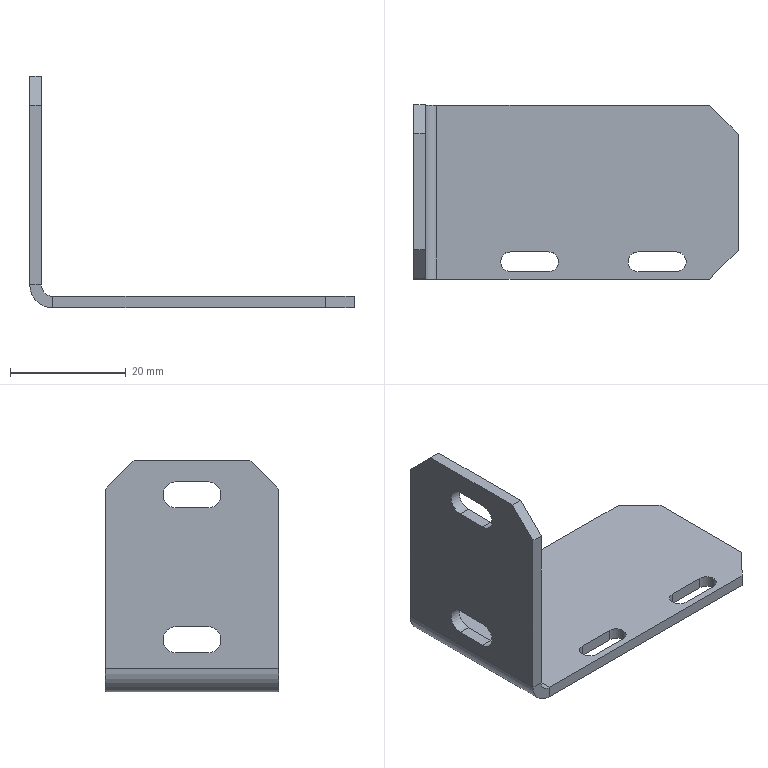Part | SolidWorks | features HoleWzd 2, Chamfer 1, EdgeFlange 1, FlatPattern 1, SMBaseFlange 1, SheetMetal 1 | 1 solid | 34 faces | box 56 x 30 x 40 mm | volume 5174 mm3 | plane 24 | cylinder 10 | commonest cylinder face diameters 3.4 x4 4.5 x4 4 x1 8 x1
STEP:
#1=CARTESIAN_POINT('',(54.,10.,-20.));
#2=VERTEX_POINT('',#1);
#3=CARTESIAN_POINT('',(54.,-10.,-20.));
#4=VERTEX_POINT('',#3);
#5=CARTESIAN_POINT('',(54.,0.,-20.));
#6=DIRECTION('',(0.,-1.,0.));
#7=VECTOR('',#6,1000.);
#8=LINE('',#5,#7);
#9=EDGE_CURVE('',#2,#4,#8,.T.);
#10=ORIENTED_EDGE('',*,*,#9,.T.);
#11=CARTESIAN_POINT('',(49.,-15.,-20.));
#12=VERTEX_POINT('',#11);
#13=CARTESIAN_POINT('',(49.,-15.,-20.));
#14=DIRECTION('',(-0.7071,-0.7071,0.));
#15=VECTOR('',#14,1000.);
#16=LINE('',#13,#15);
#17=EDGE_CURVE('',#4,#12,#16,.T.);
#18=ORIENTED_EDGE('',*,*,#17,.T.);
#19=CARTESIAN_POINT('',(2.,-15.,-20.));
#20=VERTEX_POINT('',#19);
#21=CARTESIAN_POINT('',(0.,-15.,-20.));
#22=DIRECTION('',(-1.,0.,0.));
#23=VECTOR('',#22,1000.);
#24=LINE('',#21,#23);
#25=EDGE_CURVE('',#12,#20,#24,.T.);
#26=ORIENTED_EDGE('',*,*,#25,.T.);
#27=CARTESIAN_POINT('',(2.,15.,-20.));
#28=VERTEX_POINT('',#27);
#29=CARTESIAN_POINT('',(2.,-15.,-20.));
#30=DIRECTION('',(0.,-1.,0.));
#31=VECTOR('',#30,1000.);
#32=LINE('',#29,#31);
#33=EDGE_CURVE('',#28,#20,#32,.T.);
#34=ORIENTED_EDGE('',*,*,#33,.F.);
#35=CARTESIAN_POINT('',(49.,15.,-20.));
#36=VERTEX_POINT('',#35);
#37=CARTESIAN_POINT('',(0.,15.,-20.));
#38=DIRECTION('',(1.,0.,0.));
#39=VECTOR('',#38,1000.);
#40=LINE('',#37,#39);
#41=EDGE_CURVE('',#28,#36,#40,.T.);
#42=ORIENTED_EDGE('',*,*,#41,.T.);
#43=CARTESIAN_POINT('',(54.,10.,-20.));
#44=DIRECTION('',(0.7071,-0.7071,0.));
#45=VECTOR('',#44,1000.);
#46=LINE('',#43,#45);
#47=EDGE_CURVE('',#36,#2,#46,.T.);
#48=ORIENTED_EDGE('',*,*,#47,.T.);
#49=EDGE_LOOP('',(#10,#18,#26,#34,#42,#48));
#50=FACE_OUTER_BOUND('',#49,.T.);
#51=CARTESIAN_POINT('',(21.3,-10.3,-20.));
#52=VERTEX_POINT('',#51);
#53=CARTESIAN_POINT('',(21.3,-13.7,-20.));
#54=VERTEX_POINT('',#53);
#55=CARTESIAN_POINT('',(21.3,-12.,-20.));
#56=DIRECTION('',(0.,0.,-1.));
#57=DIRECTION('',(0.,1.,0.));
#58=AXIS2_PLACEMENT_3D('',#55,#56,#57);
#59=CIRCLE('',#58,1.7);
#60=EDGE_CURVE('',#52,#54,#59,.T.);
#61=ORIENTED_EDGE('',*,*,#60,.F.);
#62=CARTESIAN_POINT('',(14.7,-10.3,-20.));
#63=VERTEX_POINT('',#62);
#64=CARTESIAN_POINT('',(21.3,-10.3,-20.));
#65=DIRECTION('',(-1.,0.,0.));
#66=VECTOR('',#65,1000.);
#67=LINE('',#64,#66);
#68=EDGE_CURVE('',#52,#63,#67,.T.);
#69=ORIENTED_EDGE('',*,*,#68,.T.);
#70=CARTESIAN_POINT('',(14.7,-13.7,-20.));
#71=VERTEX_POINT('',#70);
#72=CARTESIAN_POINT('',(14.7,-12.,-20.));
#73=DIRECTION('',(0.,0.,-1.));
#74=DIRECTION('',(0.,1.,0.));
#75=AXIS2_PLACEMENT_3D('',#72,#73,#74);
#76=CIRCLE('',#75,1.7);
#77=EDGE_CURVE('',#71,#63,#76,.T.);
#78=ORIENTED_EDGE('',*,*,#77,.F.);
#79=CARTESIAN_POINT('',(21.3,-13.7,-20.));
#80=DIRECTION('',(-1.,0.,0.));
#81=VECTOR('',#80,1000.);
#82=LINE('',#79,#81);
#83=EDGE_CURVE('',#54,#71,#82,.T.);
#84=ORIENTED_EDGE('',*,*,#83,.F.);
#85=EDGE_LOOP('',(#61,#69,#78,#84));
#86=FACE_BOUND('',#85,.T.);
#87=CARTESIAN_POINT('',(43.3,-13.7,-20.));
#88=VERTEX_POINT('',#87);
#89=CARTESIAN_POINT('',(36.7,-13.7,-20.));
#90=VERTEX_POINT('',#89);
#91=CARTESIAN_POINT('',(43.3,-13.7,-20.));
#92=DIRECTION('',(-1.,0.,0.));
#93=VECTOR('',#92,1000.);
#94=LINE('',#91,#93);
#95=EDGE_CURVE('',#88,#90,#94,.T.);
#96=ORIENTED_EDGE('',*,*,#95,.F.);
#97=CARTESIAN_POINT('',(43.3,-10.3,-20.));
#98=VERTEX_POINT('',#97);
#99=CARTESIAN_POINT('',(43.3,-12.,-20.));
#100=DIRECTION('',(0.,0.,-1.));
#101=DIRECTION('',(0.,1.,0.));
#102=AXIS2_PLACEMENT_3D('',#99,#100,#101);
#103=CIRCLE('',#102,1.7);
#104=EDGE_CURVE('',#98,#88,#103,.T.);
#105=ORIENTED_EDGE('',*,*,#104,.F.);
#106=CARTESIAN_POINT('',(36.7,-10.3,-20.));
#107=VERTEX_POINT('',#106);
#108=CARTESIAN_POINT('',(43.3,-10.3,-20.));
#109=DIRECTION('',(-1.,0.,0.));
#110=VECTOR('',#109,1000.);
#111=LINE('',#108,#110);
#112=EDGE_CURVE('',#98,#107,#111,.T.);
#113=ORIENTED_EDGE('',*,*,#112,.T.);
#114=CARTESIAN_POINT('',(36.7,-12.,-20.));
#115=DIRECTION('',(0.,0.,-1.));
#116=DIRECTION('',(0.,1.,0.));
#117=AXIS2_PLACEMENT_3D('',#114,#115,#116);
#118=CIRCLE('',#117,1.7);
#119=EDGE_CURVE('',#90,#107,#118,.T.);
#120=ORIENTED_EDGE('',*,*,#119,.F.);
#121=EDGE_LOOP('',(#96,#105,#113,#120));
#122=FACE_BOUND('',#121,.T.);
#123=CARTESIAN_POINT('',(0.,0.,-20.));
#124=DIRECTION('',(0.,0.,1.));
#125=DIRECTION('',(1.,0.,0.));
#126=AXIS2_PLACEMENT_3D('',#123,#124,#125);
#127=PLANE('',#126);
#128=ADVANCED_FACE('',(#50,#86,#122),#127,.F.);
#129=CARTESIAN_POINT('',(-2.,15.,-16.));
#130=VERTEX_POINT('',#129);
#131=CARTESIAN_POINT('',(-2.,15.,15.));
#132=VERTEX_POINT('',#131);
#133=CARTESIAN_POINT('',(-2.,15.,20.));
#134=DIRECTION('',(0.,0.,1.));
#135=VECTOR('',#134,1000.);
#136=LINE('',#133,#135);
#137=EDGE_CURVE('',#130,#132,#136,.T.);
#138=ORIENTED_EDGE('',*,*,#137,.T.);
#139=CARTESIAN_POINT('',(0.,15.,15.));
#140=VERTEX_POINT('',#139);
#141=CARTESIAN_POINT('',(-2.,15.,15.));
#142=DIRECTION('',(1.,0.,0.));
#143=VECTOR('',#142,1000.);
#144=LINE('',#141,#143);
#145=EDGE_CURVE('',#132,#140,#144,.T.);
#146=ORIENTED_EDGE('',*,*,#145,.T.);
#147=CARTESIAN_POINT('',(0.,15.,-16.));
#148=VERTEX_POINT('',#147);
#149=CARTESIAN_POINT('',(0.,15.,20.));
#150=DIRECTION('',(0.,0.,1.));
#151=VECTOR('',#150,1000.);
#152=LINE('',#149,#151);
#153=EDGE_CURVE('',#148,#140,#152,.T.);
#154=ORIENTED_EDGE('',*,*,#153,.F.);
#155=CARTESIAN_POINT('',(0.,15.,-16.));
#156=DIRECTION('',(-1.,0.,0.));
#157=VECTOR('',#156,1000.);
#158=LINE('',#155,#157);
#159=EDGE_CURVE('',#148,#130,#158,.T.);
#160=ORIENTED_EDGE('',*,*,#159,.T.);
#161=EDGE_LOOP('',(#138,#146,#154,#160));
#162=FACE_OUTER_BOUND('',#161,.T.);
#163=CARTESIAN_POINT('',(-2.,15.,20.));
#164=DIRECTION('',(0.,1.,0.));
#165=DIRECTION('',(0.,0.,1.));
#166=AXIS2_PLACEMENT_3D('',#163,#164,#165);
#167=PLANE('',#166);
#168=ADVANCED_FACE('',(#162),#167,.T.);
#169=CARTESIAN_POINT('',(-2.,2.75,16.25));
#170=VERTEX_POINT('',#169);
#171=CARTESIAN_POINT('',(-2.,-2.75,16.25));
#172=VERTEX_POINT('',#171);
#173=CARTESIAN_POINT('',(-2.,2.75,16.25));
#174=DIRECTION('',(0.,-1.,0.));
#175=VECTOR('',#174,1000.);
#176=LINE('',#173,#175);
#177=EDGE_CURVE('',#170,#172,#176,.T.);
#178=ORIENTED_EDGE('',*,*,#177,.T.);
#179=CARTESIAN_POINT('',(-2.,-2.75,11.75));
#180=VERTEX_POINT('',#179);
#181=CARTESIAN_POINT('',(-2.,-2.75,14.));
#182=DIRECTION('',(1.,0.,0.));
#183=DIRECTION('',(0.,0.,-1.));
#184=AXIS2_PLACEMENT_3D('',#181,#182,#183);
#185=CIRCLE('',#184,2.25);
#186=EDGE_CURVE('',#172,#180,#185,.T.);
#187=ORIENTED_EDGE('',*,*,#186,.T.);
#188=CARTESIAN_POINT('',(-2.,2.75,11.75));
#189=VERTEX_POINT('',#188);
#190=CARTESIAN_POINT('',(-2.,2.75,11.75));
#191=DIRECTION('',(0.,-1.,0.));
#192=VECTOR('',#191,1000.);
#193=LINE('',#190,#192);
#194=EDGE_CURVE('',#189,#180,#193,.T.);
#195=ORIENTED_EDGE('',*,*,#194,.F.);
#196=CARTESIAN_POINT('',(-2.,2.75,14.));
#197=DIRECTION('',(1.,0.,0.));
#198=DIRECTION('',(0.,0.,-1.));
#199=AXIS2_PLACEMENT_3D('',#196,#197,#198);
#200=CIRCLE('',#199,2.25);
#201=EDGE_CURVE('',#189,#170,#200,.T.);
#202=ORIENTED_EDGE('',*,*,#201,.T.);
#203=EDGE_LOOP('',(#178,#187,#195,#202));
#204=FACE_BOUND('',#203,.T.);
#205=CARTESIAN_POINT('',(-2.,2.75,-13.25));
#206=VERTEX_POINT('',#205);
#207=CARTESIAN_POINT('',(-2.,2.75,-8.75));
#208=VERTEX_POINT('',#207);
#209=CARTESIAN_POINT('',(-2.,2.75,-11.));
#210=DIRECTION('',(1.,0.,0.));
#211=DIRECTION('',(0.,0.,-1.));
#212=AXIS2_PLACEMENT_3D('',#209,#210,#211);
#213=CIRCLE('',#212,2.25);
#214=EDGE_CURVE('',#206,#208,#213,.T.);
#215=ORIENTED_EDGE('',*,*,#214,.T.);
#216=CARTESIAN_POINT('',(-2.,-2.75,-8.75));
#217=VERTEX_POINT('',#216);
#218=CARTESIAN_POINT('',(-2.,2.75,-8.75));
#219=DIRECTION('',(0.,-1.,0.));
#220=VECTOR('',#219,1000.);
#221=LINE('',#218,#220);
#222=EDGE_CURVE('',#208,#217,#221,.T.);
#223=ORIENTED_EDGE('',*,*,#222,.T.);
#224=CARTESIAN_POINT('',(-2.,-2.75,-13.25));
#225=VERTEX_POINT('',#224);
#226=CARTESIAN_POINT('',(-2.,-2.75,-11.));
#227=DIRECTION('',(1.,0.,0.));
#228=DIRECTION('',(0.,0.,-1.));
#229=AXIS2_PLACEMENT_3D('',#226,#227,#228);
#230=CIRCLE('',#229,2.25);
#231=EDGE_CURVE('',#217,#225,#230,.T.);
#232=ORIENTED_EDGE('',*,*,#231,.T.);
#233=CARTESIAN_POINT('',(-2.,2.75,-13.25));
#234=DIRECTION('',(0.,-1.,0.));
#235=VECTOR('',#234,1000.);
#236=LINE('',#233,#235);
#237=EDGE_CURVE('',#206,#225,#236,.T.);
#238=ORIENTED_EDGE('',*,*,#237,.F.);
#239=EDGE_LOOP('',(#215,#223,#232,#238));
#240=FACE_BOUND('',#239,.T.);
#241=CARTESIAN_POINT('',(-2.,-15.,15.));
#242=VERTEX_POINT('',#241);
#243=CARTESIAN_POINT('',(-2.,-15.,-16.));
#244=VERTEX_POINT('',#243);
#245=CARTESIAN_POINT('',(-2.,-15.,20.));
#246=DIRECTION('',(0.,0.,-1.));
#247=VECTOR('',#246,1000.);
#248=LINE('',#245,#247);
#249=EDGE_CURVE('',#242,#244,#248,.T.);
#250=ORIENTED_EDGE('',*,*,#249,.F.);
#251=CARTESIAN_POINT('',(-2.,-10.,20.));
#252=VERTEX_POINT('',#251);
#253=CARTESIAN_POINT('',(-2.,-10.,20.));
#254=DIRECTION('',(0.,0.7071,0.7071));
#255=VECTOR('',#254,1000.);
#256=LINE('',#253,#255);
#257=EDGE_CURVE('',#242,#252,#256,.T.);
#258=ORIENTED_EDGE('',*,*,#257,.T.);
#259=CARTESIAN_POINT('',(-2.,10.,20.));
#260=VERTEX_POINT('',#259);
#261=CARTESIAN_POINT('',(-2.,15.,20.));
#262=DIRECTION('',(0.,-1.,0.));
#263=VECTOR('',#262,1000.);
#264=LINE('',#261,#263);
#265=EDGE_CURVE('',#260,#252,#264,.T.);
#266=ORIENTED_EDGE('',*,*,#265,.F.);
#267=CARTESIAN_POINT('',(-2.,15.,15.));
#268=DIRECTION('',(0.,0.7071,-0.7071));
#269=VECTOR('',#268,1000.);
#270=LINE('',#267,#269);
#271=EDGE_CURVE('',#260,#132,#270,.T.);
#272=ORIENTED_EDGE('',*,*,#271,.T.);
#273=ORIENTED_EDGE('',*,*,#137,.F.);
#274=CARTESIAN_POINT('',(-2.,15.,-16.));
#275=DIRECTION('',(0.,-1.,0.));
#276=VECTOR('',#275,1000.);
#277=LINE('',#274,#276);
#278=EDGE_CURVE('',#130,#244,#277,.T.);
#279=ORIENTED_EDGE('',*,*,#278,.T.);
#280=EDGE_LOOP('',(#250,#258,#266,#272,#273,#279));
#281=FACE_OUTER_BOUND('',#280,.T.);
#282=CARTESIAN_POINT('',(-2.,0.,0.));
#283=DIRECTION('',(1.,0.,0.));
#284=DIRECTION('',(0.,0.,-1.));
#285=AXIS2_PLACEMENT_3D('',#282,#283,#284);
#286=PLANE('',#285);
#287=ADVANCED_FACE('',(#204,#240,#281),#286,.F.);
#288=CARTESIAN_POINT('',(0.,2.75,11.75));
#289=VERTEX_POINT('',#288);
#290=CARTESIAN_POINT('',(0.,-2.75,11.75));
#291=VERTEX_POINT('',#290);
#292=CARTESIAN_POINT('',(0.,2.75,11.75));
#293=DIRECTION('',(0.,-1.,0.));
#294=VECTOR('',#293,1000.);
#295=LINE('',#292,#294);
#296=EDGE_CURVE('',#289,#291,#295,.T.);
#297=ORIENTED_EDGE('',*,*,#296,.T.);
#298=CARTESIAN_POINT('',(0.,-2.75,16.25));
#299=VERTEX_POINT('',#298);
#300=CARTESIAN_POINT('',(0.,-2.75,14.));
#301=DIRECTION('',(1.,0.,0.));
#302=DIRECTION('',(0.,0.,-1.));
#303=AXIS2_PLACEMENT_3D('',#300,#301,#302);
#304=CIRCLE('',#303,2.25);
#305=EDGE_CURVE('',#299,#291,#304,.T.);
#306=ORIENTED_EDGE('',*,*,#305,.F.);
#307=CARTESIAN_POINT('',(0.,2.75,16.25));
#308=VERTEX_POINT('',#307);
#309=CARTESIAN_POINT('',(0.,2.75,16.25));
#310=DIRECTION('',(0.,-1.,0.));
#311=VECTOR('',#310,1000.);
#312=LINE('',#309,#311);
#313=EDGE_CURVE('',#308,#299,#312,.T.);
#314=ORIENTED_EDGE('',*,*,#313,.F.);
#315=CARTESIAN_POINT('',(0.,2.75,14.));
#316=DIRECTION('',(1.,0.,0.));
#317=DIRECTION('',(0.,0.,-1.));
#318=AXIS2_PLACEMENT_3D('',#315,#316,#317);
#319=CIRCLE('',#318,2.25);
#320=EDGE_CURVE('',#289,#308,#319,.T.);
#321=ORIENTED_EDGE('',*,*,#320,.F.);
#322=EDGE_LOOP('',(#297,#306,#314,#321));
#323=FACE_BOUND('',#322,.T.);
#324=CARTESIAN_POINT('',(0.,2.75,-13.25));
#325=VERTEX_POINT('',#324);
#326=CARTESIAN_POINT('',(0.,-2.75,-13.25));
#327=VERTEX_POINT('',#326);
#328=CARTESIAN_POINT('',(0.,2.75,-13.25));
#329=DIRECTION('',(0.,-1.,0.));
#330=VECTOR('',#329,1000.);
#331=LINE('',#328,#330);
#332=EDGE_CURVE('',#325,#327,#331,.T.);
#333=ORIENTED_EDGE('',*,*,#332,.T.);
#334=CARTESIAN_POINT('',(0.,-2.75,-8.75));
#335=VERTEX_POINT('',#334);
#336=CARTESIAN_POINT('',(0.,-2.75,-11.));
#337=DIRECTION('',(1.,0.,0.));
#338=DIRECTION('',(0.,0.,-1.));
#339=AXIS2_PLACEMENT_3D('',#336,#337,#338);
#340=CIRCLE('',#339,2.25);
#341=EDGE_CURVE('',#335,#327,#340,.T.);
#342=ORIENTED_EDGE('',*,*,#341,.F.);
#343=CARTESIAN_POINT('',(0.,2.75,-8.75));
#344=VERTEX_POINT('',#343);
#345=CARTESIAN_POINT('',(0.,2.75,-8.75));
#346=DIRECTION('',(0.,-1.,0.));
#347=VECTOR('',#346,1000.);
#348=LINE('',#345,#347);
#349=EDGE_CURVE('',#344,#335,#348,.T.);
#350=ORIENTED_EDGE('',*,*,#349,.F.);
#351=CARTESIAN_POINT('',(0.,2.75,-11.));
#352=DIRECTION('',(1.,0.,0.));
#353=DIRECTION('',(0.,0.,-1.));
#354=AXIS2_PLACEMENT_3D('',#351,#352,#353);
#355=CIRCLE('',#354,2.25);
#356=EDGE_CURVE('',#325,#344,#355,.T.);
#357=ORIENTED_EDGE('',*,*,#356,.F.);
#358=EDGE_LOOP('',(#333,#342,#350,#357));
#359=FACE_BOUND('',#358,.T.);
#360=CARTESIAN_POINT('',(0.,10.,20.));
#361=VERTEX_POINT('',#360);
#362=CARTESIAN_POINT('',(0.,-10.,20.));
#363=VERTEX_POINT('',#362);
#364=CARTESIAN_POINT('',(0.,15.,20.));
#365=DIRECTION('',(0.,-1.,0.));
#366=VECTOR('',#365,1000.);
#367=LINE('',#364,#366);
#368=EDGE_CURVE('',#361,#363,#367,.T.);
#369=ORIENTED_EDGE('',*,*,#368,.T.);
#370=CARTESIAN_POINT('',(0.,-15.,15.));
#371=VERTEX_POINT('',#370);
#372=CARTESIAN_POINT('',(0.,-15.,15.));
#373=DIRECTION('',(0.,-0.7071,-0.7071));
#374=VECTOR('',#373,1000.);
#375=LINE('',#372,#374);
#376=EDGE_CURVE('',#363,#371,#375,.T.);
#377=ORIENTED_EDGE('',*,*,#376,.T.);
#378=CARTESIAN_POINT('',(0.,-15.,-16.));
#379=VERTEX_POINT('',#378);
#380=CARTESIAN_POINT('',(0.,-15.,20.));
#381=DIRECTION('',(0.,0.,-1.));
#382=VECTOR('',#381,1000.);
#383=LINE('',#380,#382);
#384=EDGE_CURVE('',#371,#379,#383,.T.);
#385=ORIENTED_EDGE('',*,*,#384,.T.);
#386=CARTESIAN_POINT('',(0.,15.,-16.));
#387=DIRECTION('',(0.,-1.,0.));
#388=VECTOR('',#387,1000.);
#389=LINE('',#386,#388);
#390=EDGE_CURVE('',#148,#379,#389,.T.);
#391=ORIENTED_EDGE('',*,*,#390,.F.);
#392=ORIENTED_EDGE('',*,*,#153,.T.);
#393=CARTESIAN_POINT('',(0.,15.,15.));
#394=DIRECTION('',(0.,-0.7071,0.7071));
#395=VECTOR('',#394,1000.);
#396=LINE('',#393,#395);
#397=EDGE_CURVE('',#140,#361,#396,.T.);
#398=ORIENTED_EDGE('',*,*,#397,.T.);
#399=EDGE_LOOP('',(#369,#377,#385,#391,#392,#398));
#400=FACE_OUTER_BOUND('',#399,.T.);
#401=CARTESIAN_POINT('',(0.,0.,0.));
#402=DIRECTION('',(1.,0.,0.));
#403=DIRECTION('',(0.,0.,-1.));
#404=AXIS2_PLACEMENT_3D('',#401,#402,#403);
#405=PLANE('',#404);
#406=ADVANCED_FACE('',(#323,#359,#400),#405,.T.);
#407=ORIENTED_EDGE('',*,*,#384,.F.);
#408=CARTESIAN_POINT('',(-2.,-15.,15.));
#409=DIRECTION('',(-1.,0.,0.));
#410=VECTOR('',#409,1000.);
#411=LINE('',#408,#410);
#412=EDGE_CURVE('',#371,#242,#411,.T.);
#413=ORIENTED_EDGE('',*,*,#412,.T.);
#414=ORIENTED_EDGE('',*,*,#249,.T.);
#415=CARTESIAN_POINT('',(0.,-15.,-16.));
#416=DIRECTION('',(-1.,0.,0.));
#417=VECTOR('',#416,1000.);
#418=LINE('',#415,#417);
#419=EDGE_CURVE('',#379,#244,#418,.T.);
#420=ORIENTED_EDGE('',*,*,#419,.F.);
#421=EDGE_LOOP('',(#407,#413,#414,#420));
#422=FACE_OUTER_BOUND('',#421,.T.);
#423=CARTESIAN_POINT('',(-2.,-15.,20.));
#424=DIRECTION('',(0.,-1.,0.));
#425=DIRECTION('',(0.,0.,-1.));
#426=AXIS2_PLACEMENT_3D('',#423,#424,#425);
#427=PLANE('',#426);
#428=ADVANCED_FACE('',(#422),#427,.T.);
#429=ORIENTED_EDGE('',*,*,#265,.T.);
#430=CARTESIAN_POINT('',(-2.,-10.,20.));
#431=DIRECTION('',(1.,0.,0.));
#432=VECTOR('',#431,1000.);
#433=LINE('',#430,#432);
#434=EDGE_CURVE('',#252,#363,#433,.T.);
#435=ORIENTED_EDGE('',*,*,#434,.T.);
#436=ORIENTED_EDGE('',*,*,#368,.F.);
#437=CARTESIAN_POINT('',(-2.,10.,20.));
#438=DIRECTION('',(-1.,0.,0.));
#439=VECTOR('',#438,1000.);
#440=LINE('',#437,#439);
#441=EDGE_CURVE('',#361,#260,#440,.T.);
#442=ORIENTED_EDGE('',*,*,#441,.T.);
#443=EDGE_LOOP('',(#429,#435,#436,#442));
#444=FACE_OUTER_BOUND('',#443,.T.);
#445=CARTESIAN_POINT('',(-2.,15.,20.));
#446=DIRECTION('',(0.,0.,1.));
#447=DIRECTION('',(0.,-1.,0.));
#448=AXIS2_PLACEMENT_3D('',#445,#446,#447);
#449=PLANE('',#448);
#450=ADVANCED_FACE('',(#444),#449,.T.);
#451=CARTESIAN_POINT('',(2.,-15.,-18.));
#452=VERTEX_POINT('',#451);
#453=CARTESIAN_POINT('',(2.,-15.,-20.));
#454=DIRECTION('',(0.,0.,-1.));
#455=VECTOR('',#454,1000.);
#456=LINE('',#453,#455);
#457=EDGE_CURVE('',#452,#20,#456,.T.);
#458=ORIENTED_EDGE('',*,*,#457,.F.);
#459=CARTESIAN_POINT('',(2.,-15.,-16.));
#460=DIRECTION('',(0.,-1.,0.));
#461=DIRECTION('',(0.,0.,1.));
#462=AXIS2_PLACEMENT_3D('',#459,#460,#461);
#463=CIRCLE('',#462,2.);
#464=EDGE_CURVE('',#379,#452,#463,.T.);
#465=ORIENTED_EDGE('',*,*,#464,.F.);
#466=ORIENTED_EDGE('',*,*,#419,.T.);
#467=CARTESIAN_POINT('',(2.,-15.,-16.));
#468=DIRECTION('',(0.,-1.,0.));
#469=DIRECTION('',(0.,0.,1.));
#470=AXIS2_PLACEMENT_3D('',#467,#468,#469);
#471=CIRCLE('',#470,4.);
#472=EDGE_CURVE('',#244,#20,#471,.T.);
#473=ORIENTED_EDGE('',*,*,#472,.T.);
#474=EDGE_LOOP('',(#458,#465,#466,#473));
#475=FACE_OUTER_BOUND('',#474,.T.);
#476=CARTESIAN_POINT('',(2.,-15.,-16.));
#477=DIRECTION('',(0.,-1.,0.));
#478=DIRECTION('',(0.,0.,-1.));
#479=AXIS2_PLACEMENT_3D('',#476,#477,#478);
#480=PLANE('',#479);
#481=ADVANCED_FACE('',(#475),#480,.T.);
#482=CARTESIAN_POINT('',(2.,15.,-18.));
#483=VERTEX_POINT('',#482);
#484=CARTESIAN_POINT('',(2.,15.,-16.));
#485=DIRECTION('',(0.,1.,0.));
#486=DIRECTION('',(0.,0.,1.));
#487=AXIS2_PLACEMENT_3D('',#484,#485,#486);
#488=CIRCLE('',#487,2.);
#489=EDGE_CURVE('',#483,#148,#488,.T.);
#490=ORIENTED_EDGE('',*,*,#489,.F.);
#491=CARTESIAN_POINT('',(2.,15.,-18.));
#492=DIRECTION('',(0.,0.,-1.));
#493=VECTOR('',#492,1000.);
#494=LINE('',#491,#493);
#495=EDGE_CURVE('',#483,#28,#494,.T.);
#496=ORIENTED_EDGE('',*,*,#495,.T.);
#497=CARTESIAN_POINT('',(2.,15.,-16.));
#498=DIRECTION('',(0.,1.,0.));
#499=DIRECTION('',(0.,0.,1.));
#500=AXIS2_PLACEMENT_3D('',#497,#498,#499);
#501=CIRCLE('',#500,4.);
#502=EDGE_CURVE('',#28,#130,#501,.T.);
#503=ORIENTED_EDGE('',*,*,#502,.T.);
#504=ORIENTED_EDGE('',*,*,#159,.F.);
#505=EDGE_LOOP('',(#490,#496,#503,#504));
#506=FACE_OUTER_BOUND('',#505,.T.);
#507=CARTESIAN_POINT('',(2.,15.,-16.));
#508=DIRECTION('',(0.,-1.,0.));
#509=DIRECTION('',(0.,0.,-1.));
#510=AXIS2_PLACEMENT_3D('',#507,#508,#509);
#511=PLANE('',#510);
#512=ADVANCED_FACE('',(#506),#511,.F.);
#513=ORIENTED_EDGE('',*,*,#278,.F.);
#514=ORIENTED_EDGE('',*,*,#502,.F.);
#515=ORIENTED_EDGE('',*,*,#33,.T.);
#516=ORIENTED_EDGE('',*,*,#472,.F.);
#517=EDGE_LOOP('',(#513,#514,#515,#516));
#518=FACE_OUTER_BOUND('',#517,.T.);
#519=CARTESIAN_POINT('',(2.,15.,-16.));
#520=DIRECTION('',(0.,1.,0.));
#521=DIRECTION('',(0.,0.,-1.));
#522=AXIS2_PLACEMENT_3D('',#519,#520,#521);
#523=CYLINDRICAL_SURFACE('',#522,4.);
#524=ADVANCED_FACE('',(#518),#523,.T.);
#525=ORIENTED_EDGE('',*,*,#390,.T.);
#526=ORIENTED_EDGE('',*,*,#464,.T.);
#527=CARTESIAN_POINT('',(2.,-15.,-18.));
#528=DIRECTION('',(0.,1.,0.));
#529=VECTOR('',#528,1000.);
#530=LINE('',#527,#529);
#531=EDGE_CURVE('',#452,#483,#530,.T.);
#532=ORIENTED_EDGE('',*,*,#531,.T.);
#533=ORIENTED_EDGE('',*,*,#489,.T.);
#534=EDGE_LOOP('',(#525,#526,#532,#533));
#535=FACE_OUTER_BOUND('',#534,.T.);
#536=CARTESIAN_POINT('',(2.,15.,-16.));
#537=DIRECTION('',(0.,1.,0.));
#538=DIRECTION('',(0.,0.,-1.));
#539=AXIS2_PLACEMENT_3D('',#536,#537,#538);
#540=CYLINDRICAL_SURFACE('',#539,2.);
#541=ADVANCED_FACE('',(#535),#540,.F.);
#542=ORIENTED_EDGE('',*,*,#25,.F.);
#543=CARTESIAN_POINT('',(49.,-15.,-18.));
#544=VERTEX_POINT('',#543);
#545=CARTESIAN_POINT('',(49.,-15.,-20.));
#546=DIRECTION('',(0.,0.,1.));
#547=VECTOR('',#546,1000.);
#548=LINE('',#545,#547);
#549=EDGE_CURVE('',#12,#544,#548,.T.);
#550=ORIENTED_EDGE('',*,*,#549,.T.);
#551=CARTESIAN_POINT('',(0.,-15.,-18.));
#552=DIRECTION('',(-1.,0.,0.));
#553=VECTOR('',#552,1000.);
#554=LINE('',#551,#553);
#555=EDGE_CURVE('',#544,#452,#554,.T.);
#556=ORIENTED_EDGE('',*,*,#555,.T.);
#557=ORIENTED_EDGE('',*,*,#457,.T.);
#558=EDGE_LOOP('',(#542,#550,#556,#557));
#559=FACE_OUTER_BOUND('',#558,.T.);
#560=CARTESIAN_POINT('',(0.,-15.,-20.));
#561=DIRECTION('',(0.,1.,0.));
#562=DIRECTION('',(0.,0.,1.));
#563=AXIS2_PLACEMENT_3D('',#560,#561,#562);
#564=PLANE('',#563);
#565=ADVANCED_FACE('',(#559),#564,.F.);
#566=CARTESIAN_POINT('',(49.,15.,-18.));
#567=VERTEX_POINT('',#566);
#568=CARTESIAN_POINT('',(54.,15.,-18.));
#569=DIRECTION('',(1.,0.,0.));
#570=VECTOR('',#569,1000.);
#571=LINE('',#568,#570);
#572=EDGE_CURVE('',#483,#567,#571,.T.);
#573=ORIENTED_EDGE('',*,*,#572,.T.);
#574=CARTESIAN_POINT('',(49.,15.,-20.));
#575=DIRECTION('',(0.,0.,-1.));
#576=VECTOR('',#575,1000.);
#577=LINE('',#574,#576);
#578=EDGE_CURVE('',#567,#36,#577,.T.);
#579=ORIENTED_EDGE('',*,*,#578,.T.);
#580=ORIENTED_EDGE('',*,*,#41,.F.);
#581=ORIENTED_EDGE('',*,*,#495,.F.);
#582=EDGE_LOOP('',(#573,#579,#580,#581));
#583=FACE_OUTER_BOUND('',#582,.T.);
#584=CARTESIAN_POINT('',(54.,15.,-20.));
#585=DIRECTION('',(0.,-1.,0.));
#586=DIRECTION('',(0.,0.,-1.));
#587=AXIS2_PLACEMENT_3D('',#584,#585,#586);
#588=PLANE('',#587);
#589=ADVANCED_FACE('',(#583),#588,.F.);
#590=CARTESIAN_POINT('',(36.7,-10.3,-18.));
#591=VERTEX_POINT('',#590);
#592=CARTESIAN_POINT('',(36.7,-13.7,-18.));
#593=VERTEX_POINT('',#592);
#594=CARTESIAN_POINT('',(36.7,-12.,-18.));
#595=DIRECTION('',(0.,0.,1.));
#596=DIRECTION('',(1.,0.,0.));
#597=AXIS2_PLACEMENT_3D('',#594,#595,#596);
#598=CIRCLE('',#597,1.7);
#599=EDGE_CURVE('',#591,#593,#598,.T.);
#600=ORIENTED_EDGE('',*,*,#599,.F.);
#601=CARTESIAN_POINT('',(43.3,-10.3,-18.));
#602=VERTEX_POINT('',#601);
#603=CARTESIAN_POINT('',(0.,-10.3,-18.));
#604=DIRECTION('',(-1.,0.,0.));
#605=VECTOR('',#604,1000.);
#606=LINE('',#603,#605);
#607=EDGE_CURVE('',#602,#591,#606,.T.);
#608=ORIENTED_EDGE('',*,*,#607,.F.);
#609=CARTESIAN_POINT('',(43.3,-13.7,-18.));
#610=VERTEX_POINT('',#609);
#611=CARTESIAN_POINT('',(43.3,-12.,-18.));
#612=DIRECTION('',(0.,0.,1.));
#613=DIRECTION('',(1.,0.,0.));
#614=AXIS2_PLACEMENT_3D('',#611,#612,#613);
#615=CIRCLE('',#614,1.7);
#616=EDGE_CURVE('',#610,#602,#615,.T.);
#617=ORIENTED_EDGE('',*,*,#616,.F.);
#618=CARTESIAN_POINT('',(0.,-13.7,-18.));
#619=DIRECTION('',(1.,0.,0.));
#620=VECTOR('',#619,1000.);
#621=LINE('',#618,#620);
#622=EDGE_CURVE('',#593,#610,#621,.T.);
#623=ORIENTED_EDGE('',*,*,#622,.F.);
#624=EDGE_LOOP('',(#600,#608,#617,#623));
#625=FACE_BOUND('',#624,.T.);
#626=CARTESIAN_POINT('',(14.7,-13.7,-18.));
#627=VERTEX_POINT('',#626);
#628=CARTESIAN_POINT('',(21.3,-13.7,-18.));
#629=VERTEX_POINT('',#628);
#630=CARTESIAN_POINT('',(0.,-13.7,-18.));
#631=DIRECTION('',(1.,0.,0.));
#632=VECTOR('',#631,1000.);
#633=LINE('',#630,#632);
#634=EDGE_CURVE('',#627,#629,#633,.T.);
#635=ORIENTED_EDGE('',*,*,#634,.F.);
#636=CARTESIAN_POINT('',(14.7,-10.3,-18.));
#637=VERTEX_POINT('',#636);
#638=CARTESIAN_POINT('',(14.7,-12.,-18.));
#639=DIRECTION('',(0.,0.,1.));
#640=DIRECTION('',(1.,0.,0.));
#641=AXIS2_PLACEMENT_3D('',#638,#639,#640);
#642=CIRCLE('',#641,1.7);
#643=EDGE_CURVE('',#637,#627,#642,.T.);
#644=ORIENTED_EDGE('',*,*,#643,.F.);
#645=CARTESIAN_POINT('',(21.3,-10.3,-18.));
#646=VERTEX_POINT('',#645);
#647=CARTESIAN_POINT('',(0.,-10.3,-18.));
#648=DIRECTION('',(-1.,0.,0.));
#649=VECTOR('',#648,1000.);
#650=LINE('',#647,#649);
#651=EDGE_CURVE('',#646,#637,#650,.T.);
#652=ORIENTED_EDGE('',*,*,#651,.F.);
#653=CARTESIAN_POINT('',(21.3,-12.,-18.));
#654=DIRECTION('',(0.,0.,1.));
#655=DIRECTION('',(1.,0.,0.));
#656=AXIS2_PLACEMENT_3D('',#653,#654,#655);
#657=CIRCLE('',#656,1.7);
#658=EDGE_CURVE('',#629,#646,#657,.T.);
#659=ORIENTED_EDGE('',*,*,#658,.F.);
#660=EDGE_LOOP('',(#635,#644,#652,#659));
#661=FACE_BOUND('',#660,.T.);
#662=ORIENTED_EDGE('',*,*,#555,.F.);
#663=CARTESIAN_POINT('',(54.,-10.,-18.));
#664=VERTEX_POINT('',#663);
#665=CARTESIAN_POINT('',(32.,-32.,-18.));
#666=DIRECTION('',(0.7071,0.7071,0.));
#667=VECTOR('',#666,1000.);
#668=LINE('',#665,#667);
#669=EDGE_CURVE('',#544,#664,#668,.T.);
#670=ORIENTED_EDGE('',*,*,#669,.T.);
#671=CARTESIAN_POINT('',(54.,10.,-18.));
#672=VERTEX_POINT('',#671);
#673=CARTESIAN_POINT('',(54.,-15.,-18.));
#674=DIRECTION('',(0.,-1.,0.));
#675=VECTOR('',#674,1000.);
#676=LINE('',#673,#675);
#677=EDGE_CURVE('',#672,#664,#676,.T.);
#678=ORIENTED_EDGE('',*,*,#677,.F.);
#679=CARTESIAN_POINT('',(32.,32.,-18.));
#680=DIRECTION('',(-0.7071,0.7071,0.));
#681=VECTOR('',#680,1000.);
#682=LINE('',#679,#681);
#683=EDGE_CURVE('',#672,#567,#682,.T.);
#684=ORIENTED_EDGE('',*,*,#683,.T.);
#685=ORIENTED_EDGE('',*,*,#572,.F.);
#686=ORIENTED_EDGE('',*,*,#531,.F.);
#687=EDGE_LOOP('',(#662,#670,#678,#684,#685,#686));
#688=FACE_OUTER_BOUND('',#687,.T.);
#689=CARTESIAN_POINT('',(0.,0.,-18.));
#690=DIRECTION('',(0.,0.,1.));
#691=DIRECTION('',(1.,0.,0.));
#692=AXIS2_PLACEMENT_3D('',#689,#690,#691);
#693=PLANE('',#692);
#694=ADVANCED_FACE('',(#625,#661,#688),#693,.T.);
#695=ORIENTED_EDGE('',*,*,#677,.T.);
#696=CARTESIAN_POINT('',(54.,-10.,-20.));
#697=DIRECTION('',(0.,0.,-1.));
#698=VECTOR('',#697,1000.);
#699=LINE('',#696,#698);
#700=EDGE_CURVE('',#664,#4,#699,.T.);
#701=ORIENTED_EDGE('',*,*,#700,.T.);
#702=ORIENTED_EDGE('',*,*,#9,.F.);
#703=CARTESIAN_POINT('',(54.,10.,-20.));
#704=DIRECTION('',(0.,0.,1.));
#705=VECTOR('',#704,1000.);
#706=LINE('',#703,#705);
#707=EDGE_CURVE('',#2,#672,#706,.T.);
#708=ORIENTED_EDGE('',*,*,#707,.T.);
#709=EDGE_LOOP('',(#695,#701,#702,#708));
#710=FACE_OUTER_BOUND('',#709,.T.);
#711=CARTESIAN_POINT('',(54.,-15.,-20.));
#712=DIRECTION('',(-1.,0.,0.));
#713=DIRECTION('',(0.,0.,1.));
#714=AXIS2_PLACEMENT_3D('',#711,#712,#713);
#715=PLANE('',#714);
#716=ADVANCED_FACE('',(#710),#715,.F.);
#717=ORIENTED_EDGE('',*,*,#257,.F.);
#718=ORIENTED_EDGE('',*,*,#412,.F.);
#719=ORIENTED_EDGE('',*,*,#376,.F.);
#720=ORIENTED_EDGE('',*,*,#434,.F.);
#721=EDGE_LOOP('',(#717,#718,#719,#720));
#722=FACE_OUTER_BOUND('',#721,.T.);
#723=CARTESIAN_POINT('',(-2.,-10.,20.));
#724=DIRECTION('',(0.,0.7071,-0.7071));
#725=DIRECTION('',(1.,0.,0.));
#726=AXIS2_PLACEMENT_3D('',#723,#724,#725);
#727=PLANE('',#726);
#728=ADVANCED_FACE('',(#722),#727,.F.);
#729=ORIENTED_EDGE('',*,*,#271,.F.);
#730=ORIENTED_EDGE('',*,*,#441,.F.);
#731=ORIENTED_EDGE('',*,*,#397,.F.);
#732=ORIENTED_EDGE('',*,*,#145,.F.);
#733=EDGE_LOOP('',(#729,#730,#731,#732));
#734=FACE_OUTER_BOUND('',#733,.T.);
#735=CARTESIAN_POINT('',(-2.,15.,15.));
#736=DIRECTION('',(0.,-0.7071,-0.7071));
#737=DIRECTION('',(1.,0.,0.));
#738=AXIS2_PLACEMENT_3D('',#735,#736,#737);
#739=PLANE('',#738);
#740=ADVANCED_FACE('',(#734),#739,.F.);
#741=ORIENTED_EDGE('',*,*,#17,.F.);
#742=ORIENTED_EDGE('',*,*,#700,.F.);
#743=ORIENTED_EDGE('',*,*,#669,.F.);
#744=ORIENTED_EDGE('',*,*,#549,.F.);
#745=EDGE_LOOP('',(#741,#742,#743,#744));
#746=FACE_OUTER_BOUND('',#745,.T.);
#747=CARTESIAN_POINT('',(49.,-15.,-20.));
#748=DIRECTION('',(-0.7071,0.7071,0.));
#749=DIRECTION('',(0.,0.,1.));
#750=AXIS2_PLACEMENT_3D('',#747,#748,#749);
#751=PLANE('',#750);
#752=ADVANCED_FACE('',(#746),#751,.F.);
#753=ORIENTED_EDGE('',*,*,#47,.F.);
#754=ORIENTED_EDGE('',*,*,#578,.F.);
#755=ORIENTED_EDGE('',*,*,#683,.F.);
#756=ORIENTED_EDGE('',*,*,#707,.F.);
#757=EDGE_LOOP('',(#753,#754,#755,#756));
#758=FACE_OUTER_BOUND('',#757,.T.);
#759=CARTESIAN_POINT('',(54.,10.,-20.));
#760=DIRECTION('',(-0.7071,-0.7071,0.));
#761=DIRECTION('',(0.,0.,1.));
#762=AXIS2_PLACEMENT_3D('',#759,#760,#761);
#763=PLANE('',#762);
#764=ADVANCED_FACE('',(#758),#763,.F.);
#765=ORIENTED_EDGE('',*,*,#341,.T.);
#766=CARTESIAN_POINT('',(0.,-2.75,-13.25));
#767=DIRECTION('',(1.,0.,0.));
#768=VECTOR('',#767,1000.);
#769=LINE('',#766,#768);
#770=EDGE_CURVE('',#225,#327,#769,.T.);
#771=ORIENTED_EDGE('',*,*,#770,.F.);
#772=ORIENTED_EDGE('',*,*,#231,.F.);
#773=CARTESIAN_POINT('',(0.,-2.75,-8.75));
#774=DIRECTION('',(-1.,0.,0.));
#775=VECTOR('',#774,1000.);
#776=LINE('',#773,#775);
#777=EDGE_CURVE('',#335,#217,#776,.T.);
#778=ORIENTED_EDGE('',*,*,#777,.F.);
#779=EDGE_LOOP('',(#765,#771,#772,#778));
#780=FACE_OUTER_BOUND('',#779,.T.);
#781=CARTESIAN_POINT('',(0.,-2.75,-11.));
#782=DIRECTION('',(1.,0.,0.));
#783=DIRECTION('',(0.,0.,-1.));
#784=AXIS2_PLACEMENT_3D('',#781,#782,#783);
#785=CYLINDRICAL_SURFACE('',#784,2.25);
#786=ADVANCED_FACE('',(#780),#785,.F.);
#787=ORIENTED_EDGE('',*,*,#356,.T.);
#788=CARTESIAN_POINT('',(0.,2.75,-8.75));
#789=DIRECTION('',(1.,0.,0.));
#790=VECTOR('',#789,1000.);
#791=LINE('',#788,#790);
#792=EDGE_CURVE('',#208,#344,#791,.T.);
#793=ORIENTED_EDGE('',*,*,#792,.F.);
#794=ORIENTED_EDGE('',*,*,#214,.F.);
#795=CARTESIAN_POINT('',(0.,2.75,-13.25));
#796=DIRECTION('',(-1.,0.,0.));
#797=VECTOR('',#796,1000.);
#798=LINE('',#795,#797);
#799=EDGE_CURVE('',#325,#206,#798,.T.);
#800=ORIENTED_EDGE('',*,*,#799,.F.);
#801=EDGE_LOOP('',(#787,#793,#794,#800));
#802=FACE_OUTER_BOUND('',#801,.T.);
#803=CARTESIAN_POINT('',(0.,2.75,-11.));
#804=DIRECTION('',(1.,0.,0.));
#805=DIRECTION('',(0.,0.,-1.));
#806=AXIS2_PLACEMENT_3D('',#803,#804,#805);
#807=CYLINDRICAL_SURFACE('',#806,2.25);
#808=ADVANCED_FACE('',(#802),#807,.F.);
#809=ORIENTED_EDGE('',*,*,#770,.T.);
#810=ORIENTED_EDGE('',*,*,#332,.F.);
#811=ORIENTED_EDGE('',*,*,#799,.T.);
#812=ORIENTED_EDGE('',*,*,#237,.T.);
#813=EDGE_LOOP('',(#809,#810,#811,#812));
#814=FACE_OUTER_BOUND('',#813,.T.);
#815=CARTESIAN_POINT('',(0.,2.75,-13.25));
#816=DIRECTION('',(0.,0.,-1.));
#817=DIRECTION('',(-1.,0.,0.));
#818=AXIS2_PLACEMENT_3D('',#815,#816,#817);
#819=PLANE('',#818);
#820=ADVANCED_FACE('',(#814),#819,.F.);
#821=ORIENTED_EDGE('',*,*,#777,.T.);
#822=ORIENTED_EDGE('',*,*,#222,.F.);
#823=ORIENTED_EDGE('',*,*,#792,.T.);
#824=ORIENTED_EDGE('',*,*,#349,.T.);
#825=EDGE_LOOP('',(#821,#822,#823,#824));
#826=FACE_OUTER_BOUND('',#825,.T.);
#827=CARTESIAN_POINT('',(0.,2.75,-8.75));
#828=DIRECTION('',(0.,0.,1.));
#829=DIRECTION('',(1.,0.,0.));
#830=AXIS2_PLACEMENT_3D('',#827,#828,#829);
#831=PLANE('',#830);
#832=ADVANCED_FACE('',(#826),#831,.F.);
#833=ORIENTED_EDGE('',*,*,#305,.T.);
#834=CARTESIAN_POINT('',(0.,-2.75,11.75));
#835=DIRECTION('',(1.,0.,0.));
#836=VECTOR('',#835,1000.);
#837=LINE('',#834,#836);
#838=EDGE_CURVE('',#180,#291,#837,.T.);
#839=ORIENTED_EDGE('',*,*,#838,.F.);
#840=ORIENTED_EDGE('',*,*,#186,.F.);
#841=CARTESIAN_POINT('',(0.,-2.75,16.25));
#842=DIRECTION('',(-1.,0.,0.));
#843=VECTOR('',#842,1000.);
#844=LINE('',#841,#843);
#845=EDGE_CURVE('',#299,#172,#844,.T.);
#846=ORIENTED_EDGE('',*,*,#845,.F.);
#847=EDGE_LOOP('',(#833,#839,#840,#846));
#848=FACE_OUTER_BOUND('',#847,.T.);
#849=CARTESIAN_POINT('',(0.,-2.75,14.));
#850=DIRECTION('',(1.,0.,0.));
#851=DIRECTION('',(0.,0.,-1.));
#852=AXIS2_PLACEMENT_3D('',#849,#850,#851);
#853=CYLINDRICAL_SURFACE('',#852,2.25);
#854=ADVANCED_FACE('',(#848),#853,.F.);
#855=ORIENTED_EDGE('',*,*,#320,.T.);
#856=CARTESIAN_POINT('',(0.,2.75,16.25));
#857=DIRECTION('',(1.,0.,0.));
#858=VECTOR('',#857,1000.);
#859=LINE('',#856,#858);
#860=EDGE_CURVE('',#170,#308,#859,.T.);
#861=ORIENTED_EDGE('',*,*,#860,.F.);
#862=ORIENTED_EDGE('',*,*,#201,.F.);
#863=CARTESIAN_POINT('',(0.,2.75,11.75));
#864=DIRECTION('',(-1.,0.,0.));
#865=VECTOR('',#864,1000.);
#866=LINE('',#863,#865);
#867=EDGE_CURVE('',#289,#189,#866,.T.);
#868=ORIENTED_EDGE('',*,*,#867,.F.);
#869=EDGE_LOOP('',(#855,#861,#862,#868));
#870=FACE_OUTER_BOUND('',#869,.T.);
#871=CARTESIAN_POINT('',(0.,2.75,14.));
#872=DIRECTION('',(1.,0.,0.));
#873=DIRECTION('',(0.,0.,-1.));
#874=AXIS2_PLACEMENT_3D('',#871,#872,#873);
#875=CYLINDRICAL_SURFACE('',#874,2.25);
#876=ADVANCED_FACE('',(#870),#875,.F.);
#877=ORIENTED_EDGE('',*,*,#838,.T.);
#878=ORIENTED_EDGE('',*,*,#296,.F.);
#879=ORIENTED_EDGE('',*,*,#867,.T.);
#880=ORIENTED_EDGE('',*,*,#194,.T.);
#881=EDGE_LOOP('',(#877,#878,#879,#880));
#882=FACE_OUTER_BOUND('',#881,.T.);
#883=CARTESIAN_POINT('',(0.,2.75,11.75));
#884=DIRECTION('',(0.,0.,-1.));
#885=DIRECTION('',(-1.,0.,0.));
#886=AXIS2_PLACEMENT_3D('',#883,#884,#885);
#887=PLANE('',#886);
#888=ADVANCED_FACE('',(#882),#887,.F.);
#889=ORIENTED_EDGE('',*,*,#845,.T.);
#890=ORIENTED_EDGE('',*,*,#177,.F.);
#891=ORIENTED_EDGE('',*,*,#860,.T.);
#892=ORIENTED_EDGE('',*,*,#313,.T.);
#893=EDGE_LOOP('',(#889,#890,#891,#892));
#894=FACE_OUTER_BOUND('',#893,.T.);
#895=CARTESIAN_POINT('',(0.,2.75,16.25));
#896=DIRECTION('',(0.,0.,1.));
#897=DIRECTION('',(1.,0.,0.));
#898=AXIS2_PLACEMENT_3D('',#895,#896,#897);
#899=PLANE('',#898);
#900=ADVANCED_FACE('',(#894),#899,.F.);
#901=ORIENTED_EDGE('',*,*,#643,.T.);
#902=CARTESIAN_POINT('',(14.7,-13.7,-20.));
#903=DIRECTION('',(0.,0.,1.));
#904=VECTOR('',#903,1000.);
#905=LINE('',#902,#904);
#906=EDGE_CURVE('',#71,#627,#905,.T.);
#907=ORIENTED_EDGE('',*,*,#906,.F.);
#908=ORIENTED_EDGE('',*,*,#77,.T.);
#909=CARTESIAN_POINT('',(14.7,-10.3,-20.));
#910=DIRECTION('',(0.,0.,-1.));
#911=VECTOR('',#910,1000.);
#912=LINE('',#909,#911);
#913=EDGE_CURVE('',#637,#63,#912,.T.);
#914=ORIENTED_EDGE('',*,*,#913,.F.);
#915=EDGE_LOOP('',(#901,#907,#908,#914));
#916=FACE_OUTER_BOUND('',#915,.T.);
#917=CARTESIAN_POINT('',(14.7,-12.,-20.));
#918=DIRECTION('',(0.,0.,-1.));
#919=DIRECTION('',(0.,1.,0.));
#920=AXIS2_PLACEMENT_3D('',#917,#918,#919);
#921=CYLINDRICAL_SURFACE('',#920,1.7);
#922=ADVANCED_FACE('',(#916),#921,.F.);
#923=ORIENTED_EDGE('',*,*,#658,.T.);
#924=CARTESIAN_POINT('',(21.3,-10.3,-20.));
#925=DIRECTION('',(0.,0.,1.));
#926=VECTOR('',#925,1000.);
#927=LINE('',#924,#926);
#928=EDGE_CURVE('',#52,#646,#927,.T.);
#929=ORIENTED_EDGE('',*,*,#928,.F.);
#930=ORIENTED_EDGE('',*,*,#60,.T.);
#931=CARTESIAN_POINT('',(21.3,-13.7,-20.));
#932=DIRECTION('',(0.,0.,-1.));
#933=VECTOR('',#932,1000.);
#934=LINE('',#931,#933);
#935=EDGE_CURVE('',#629,#54,#934,.T.);
#936=ORIENTED_EDGE('',*,*,#935,.F.);
#937=EDGE_LOOP('',(#923,#929,#930,#936));
#938=FACE_OUTER_BOUND('',#937,.T.);
#939=CARTESIAN_POINT('',(21.3,-12.,-20.));
#940=DIRECTION('',(0.,0.,-1.));
#941=DIRECTION('',(0.,1.,0.));
#942=AXIS2_PLACEMENT_3D('',#939,#940,#941);
#943=CYLINDRICAL_SURFACE('',#942,1.7);
#944=ADVANCED_FACE('',(#938),#943,.F.);
#945=ORIENTED_EDGE('',*,*,#651,.T.);
#946=ORIENTED_EDGE('',*,*,#913,.T.);
#947=ORIENTED_EDGE('',*,*,#68,.F.);
#948=ORIENTED_EDGE('',*,*,#928,.T.);
#949=EDGE_LOOP('',(#945,#946,#947,#948));
#950=FACE_OUTER_BOUND('',#949,.T.);
#951=CARTESIAN_POINT('',(21.3,-10.3,-20.));
#952=DIRECTION('',(0.,1.,0.));
#953=DIRECTION('',(0.,0.,1.));
#954=AXIS2_PLACEMENT_3D('',#951,#952,#953);
#955=PLANE('',#954);
#956=ADVANCED_FACE('',(#950),#955,.F.);
#957=ORIENTED_EDGE('',*,*,#634,.T.);
#958=ORIENTED_EDGE('',*,*,#935,.T.);
#959=ORIENTED_EDGE('',*,*,#83,.T.);
#960=ORIENTED_EDGE('',*,*,#906,.T.);
#961=EDGE_LOOP('',(#957,#958,#959,#960));
#962=FACE_OUTER_BOUND('',#961,.T.);
#963=CARTESIAN_POINT('',(21.3,-13.7,-20.));
#964=DIRECTION('',(0.,-1.,0.));
#965=DIRECTION('',(0.,0.,-1.));
#966=AXIS2_PLACEMENT_3D('',#963,#964,#965);
#967=PLANE('',#966);
#968=ADVANCED_FACE('',(#962),#967,.F.);
#969=ORIENTED_EDGE('',*,*,#599,.T.);
#970=CARTESIAN_POINT('',(36.7,-13.7,-20.));
#971=DIRECTION('',(0.,0.,1.));
#972=VECTOR('',#971,1000.);
#973=LINE('',#970,#972);
#974=EDGE_CURVE('',#90,#593,#973,.T.);
#975=ORIENTED_EDGE('',*,*,#974,.F.);
#976=ORIENTED_EDGE('',*,*,#119,.T.);
#977=CARTESIAN_POINT('',(36.7,-10.3,-20.));
#978=DIRECTION('',(0.,0.,-1.));
#979=VECTOR('',#978,1000.);
#980=LINE('',#977,#979);
#981=EDGE_CURVE('',#591,#107,#980,.T.);
#982=ORIENTED_EDGE('',*,*,#981,.F.);
#983=EDGE_LOOP('',(#969,#975,#976,#982));
#984=FACE_OUTER_BOUND('',#983,.T.);
#985=CARTESIAN_POINT('',(36.7,-12.,-20.));
#986=DIRECTION('',(0.,0.,-1.));
#987=DIRECTION('',(0.,1.,0.));
#988=AXIS2_PLACEMENT_3D('',#985,#986,#987);
#989=CYLINDRICAL_SURFACE('',#988,1.7);
#990=ADVANCED_FACE('',(#984),#989,.F.);
#991=ORIENTED_EDGE('',*,*,#616,.T.);
#992=CARTESIAN_POINT('',(43.3,-10.3,-20.));
#993=DIRECTION('',(0.,0.,1.));
#994=VECTOR('',#993,1000.);
#995=LINE('',#992,#994);
#996=EDGE_CURVE('',#98,#602,#995,.T.);
#997=ORIENTED_EDGE('',*,*,#996,.F.);
#998=ORIENTED_EDGE('',*,*,#104,.T.);
#999=CARTESIAN_POINT('',(43.3,-13.7,-20.));
#1000=DIRECTION('',(0.,0.,-1.));
#1001=VECTOR('',#1000,1000.);
#1002=LINE('',#999,#1001);
#1003=EDGE_CURVE('',#610,#88,#1002,.T.);
#1004=ORIENTED_EDGE('',*,*,#1003,.F.);
#1005=EDGE_LOOP('',(#991,#997,#998,#1004));
#1006=FACE_OUTER_BOUND('',#1005,.T.);
#1007=CARTESIAN_POINT('',(43.3,-12.,-20.));
#1008=DIRECTION('',(0.,0.,-1.));
#1009=DIRECTION('',(0.,1.,0.));
#1010=AXIS2_PLACEMENT_3D('',#1007,#1008,#1009);
#1011=CYLINDRICAL_SURFACE('',#1010,1.7);
#1012=ADVANCED_FACE('',(#1006),#1011,.F.);
#1013=ORIENTED_EDGE('',*,*,#607,.T.);
#1014=ORIENTED_EDGE('',*,*,#981,.T.);
#1015=ORIENTED_EDGE('',*,*,#112,.F.);
#1016=ORIENTED_EDGE('',*,*,#996,.T.);
#1017=EDGE_LOOP('',(#1013,#1014,#1015,#1016));
#1018=FACE_OUTER_BOUND('',#1017,.T.);
#1019=CARTESIAN_POINT('',(43.3,-10.3,-20.));
#1020=DIRECTION('',(0.,1.,0.));
#1021=DIRECTION('',(0.,0.,1.));
#1022=AXIS2_PLACEMENT_3D('',#1019,#1020,#1021);
#1023=PLANE('',#1022);
#1024=ADVANCED_FACE('',(#1018),#1023,.F.);
#1025=ORIENTED_EDGE('',*,*,#622,.T.);
#1026=ORIENTED_EDGE('',*,*,#1003,.T.);
#1027=ORIENTED_EDGE('',*,*,#95,.T.);
#1028=ORIENTED_EDGE('',*,*,#974,.T.);
#1029=EDGE_LOOP('',(#1025,#1026,#1027,#1028));
#1030=FACE_OUTER_BOUND('',#1029,.T.);
#1031=CARTESIAN_POINT('',(43.3,-13.7,-20.));
#1032=DIRECTION('',(0.,-1.,0.));
#1033=DIRECTION('',(0.,0.,-1.));
#1034=AXIS2_PLACEMENT_3D('',#1031,#1032,#1033);
#1035=PLANE('',#1034);
#1036=ADVANCED_FACE('',(#1030),#1035,.F.);
#1037=CLOSED_SHELL('',(#128,#168,#287,#406,#428,#450,#481,#512,#524,#541,#565,#589,#694,#716,#728,#740,#752,#764,#786,#808,#820,#832,#854,#876,#888,#900,#922,#944,#956,#968,#990,#1012,#1024,#1036));
#1038=MANIFOLD_SOLID_BREP('',#1037);
#1039=CARTESIAN_POINT('',(0.,0.,0.));
#1040=DIRECTION('',(0.,0.,1.));
#1041=DIRECTION('',(1.,0.,0.));
#1042=AXIS2_PLACEMENT_3D('',#1039,#1040,#1041);
#1043=(LENGTH_UNIT()NAMED_UNIT(*)SI_UNIT(.MILLI.,.METRE.));
#1044=UNCERTAINTY_MEASURE_WITH_UNIT(LENGTH_MEASURE(0.00001),#1043,'','');
#1045=(NAMED_UNIT(*)PLANE_ANGLE_UNIT()SI_UNIT($,.RADIAN.));
#1046=(NAMED_UNIT(*)SI_UNIT($,.STERADIAN.)SOLID_ANGLE_UNIT());
#1047=(GEOMETRIC_REPRESENTATION_CONTEXT(3)GLOBAL_UNCERTAINTY_ASSIGNED_CONTEXT((#1044))GLOBAL_UNIT_ASSIGNED_CONTEXT((#1043,#1045,#1046))REPRESENTATION_CONTEXT('',''));
#1048=ADVANCED_BREP_SHAPE_REPRESENTATION('',(#1038,#1042),#1047);